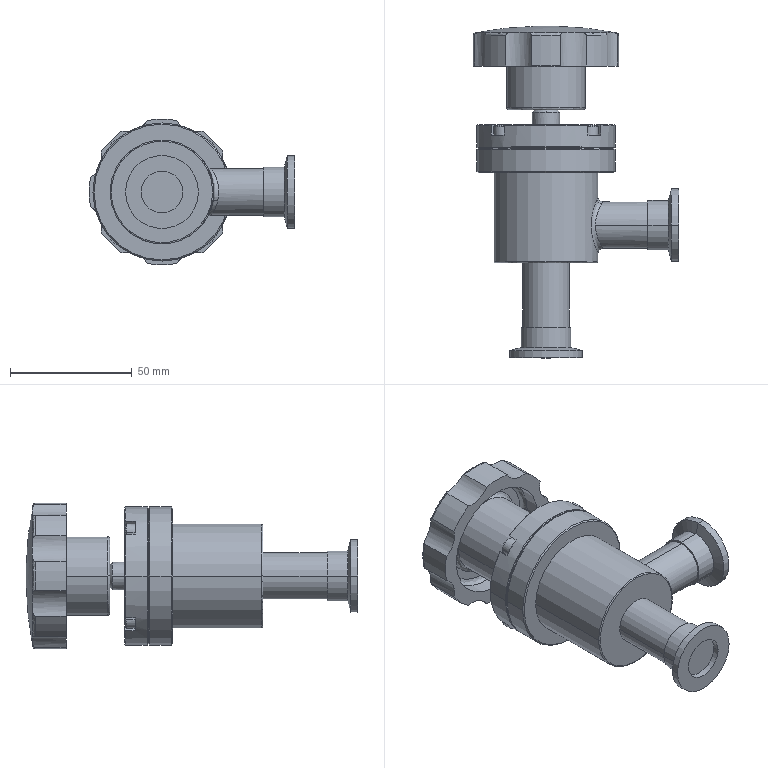Part | SolidWorks | features BaseBody 1 | 1 solid | 142 faces | box 84.6 x 136.5 x 60.001 mm | volume 174648 mm3 | cylinder 61 | plane 34 | cone 27 | spline 20 | commonest cylinder face diameters 18 x10 60.001 x9 7 x8 7.5 x6 17.2 x4 19.1 x4